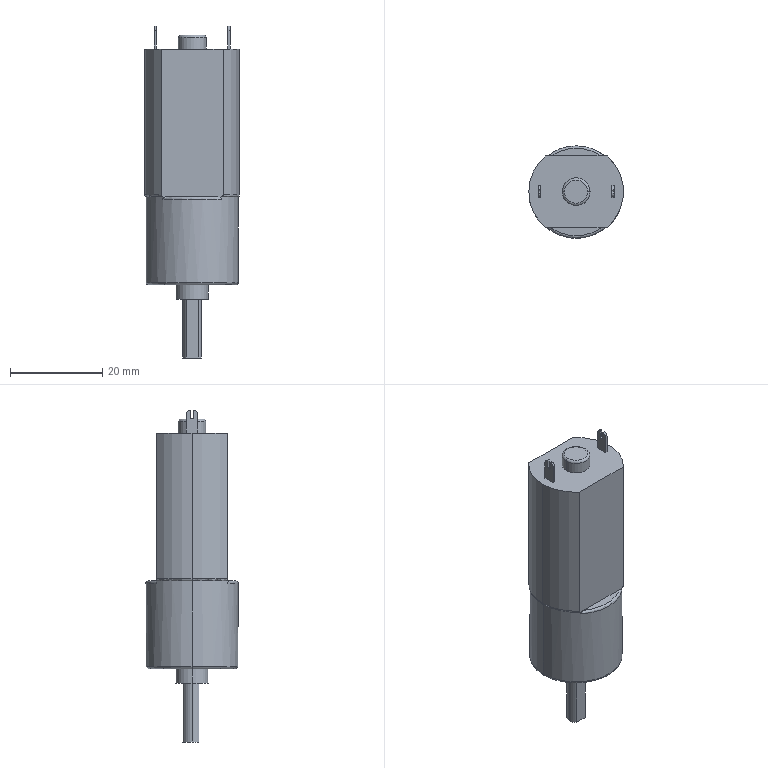Part | SolidWorks | features ICE 8, Fillet 4, MirrorPattern 3, Extrusion 1 | 1 solid | 56 faces | box 20.5 x 20 x 71.9 mm | volume 15341 mm3 | plane 24 | cylinder 23 | torus 9 | commonest cylinder face diameters 2 x8 0.75 x3 4 x3 20.5 x3 6 x2 7 x2